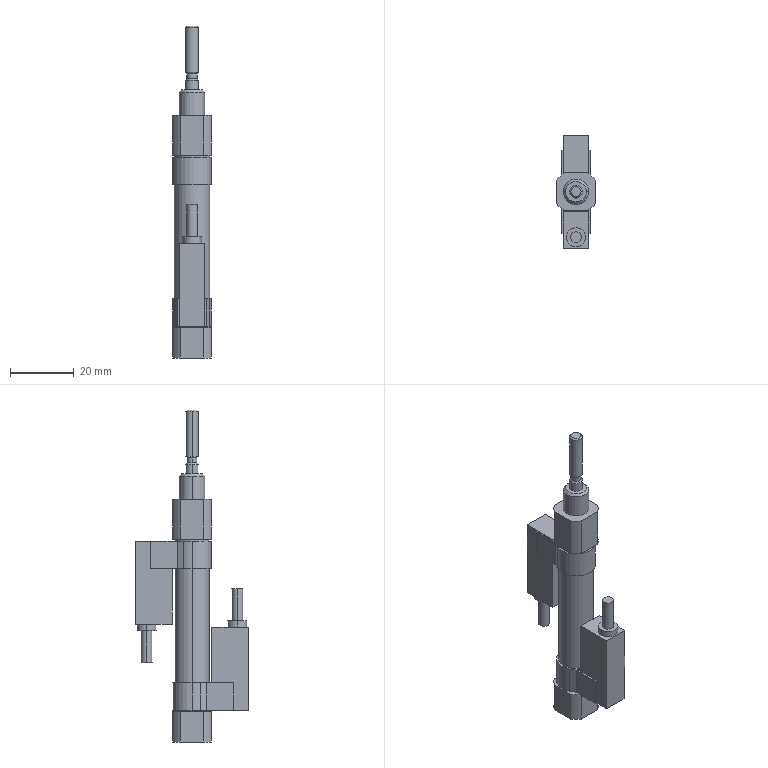Part | STEP file | CDJ2B10_30_C76_0_ | 1 solid | 106 faces | box 12.2 x 35.4 x 104 mm | volume 14245 mm3 | plane 52 | cylinder 42 | cone 12 | commonest cylinder face diameters 12.2 x8 14 x8 11 x6 3.4 x4 4 x4 4.13 x4